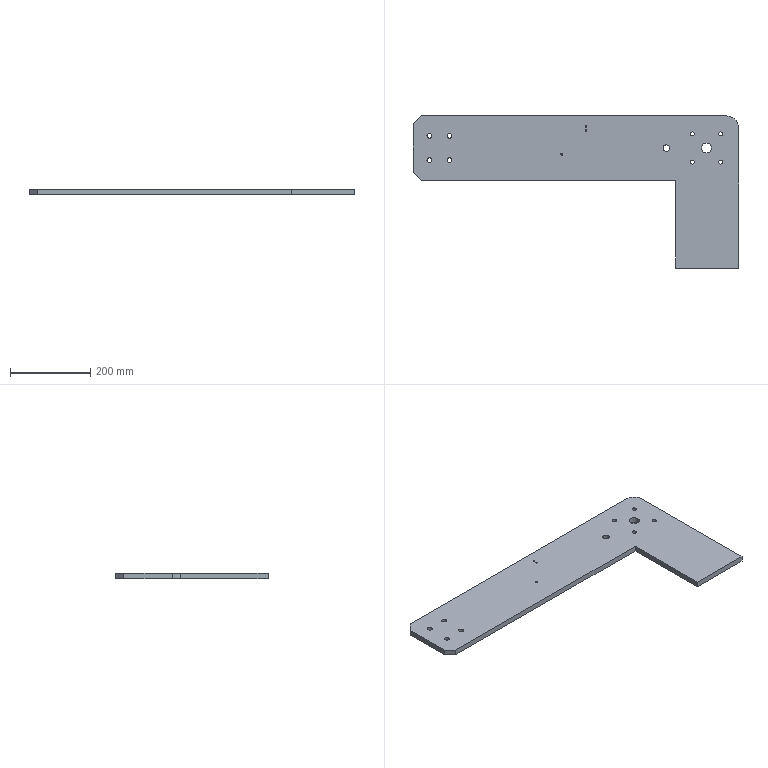Part | STEP file | Head plate 1 | 1 solid | 37 faces | box 810 x 379.049 x 14 mm | volume 2266923 mm3 | cylinder 27 | plane 10 | commonest cylinder face diameters 10 x8 12 x8 4 x4 5 x2 16 x2 25 x2
STEP:
#1=CARTESIAN_POINT('',(312.5,0.,14.));
#2=VERTEX_POINT('',#1);
#3=CARTESIAN_POINT('',(337.5,0.,14.));
#4=VERTEX_POINT('',#3);
#5=CARTESIAN_POINT('',(325.,0.,14.));
#6=DIRECTION('',(0.,0.,1.));
#7=DIRECTION('',(-1.,0.,0.));
#8=AXIS2_PLACEMENT_3D('',#5,#6,#7);
#9=CIRCLE('',#8,12.5);
#10=EDGE_CURVE('',#2,#4,#9,.T.);
#11=ORIENTED_EDGE('',*,*,#10,.T.);
#12=CARTESIAN_POINT('',(337.5,0.,0.));
#13=VERTEX_POINT('',#12);
#14=CARTESIAN_POINT('',(337.5,0.,14.));
#15=DIRECTION('',(0.,0.,-1.));
#16=VECTOR('',#15,1000.);
#17=LINE('',#14,#16);
#18=EDGE_CURVE('',#4,#13,#17,.T.);
#19=ORIENTED_EDGE('',*,*,#18,.T.);
#20=CARTESIAN_POINT('',(312.5,0.,0.));
#21=VERTEX_POINT('',#20);
#22=CARTESIAN_POINT('',(325.,0.,0.));
#23=DIRECTION('',(0.,0.,1.));
#24=DIRECTION('',(-1.,0.,0.));
#25=AXIS2_PLACEMENT_3D('',#22,#23,#24);
#26=CIRCLE('',#25,12.5);
#27=EDGE_CURVE('',#21,#13,#26,.T.);
#28=ORIENTED_EDGE('',*,*,#27,.F.);
#29=CARTESIAN_POINT('',(312.5,0.,14.));
#30=DIRECTION('',(0.,0.,-1.));
#31=VECTOR('',#30,1000.);
#32=LINE('',#29,#31);
#33=EDGE_CURVE('',#2,#21,#32,.T.);
#34=ORIENTED_EDGE('',*,*,#33,.F.);
#35=EDGE_LOOP('',(#11,#19,#28,#34));
#36=FACE_OUTER_BOUND('',#35,.T.);
#37=CARTESIAN_POINT('',(325.,0.,14.));
#38=DIRECTION('',(0.,0.,-1.));
#39=DIRECTION('',(-1.,0.,0.));
#40=AXIS2_PLACEMENT_3D('',#37,#38,#39);
#41=CYLINDRICAL_SURFACE('',#40,12.5);
#42=ADVANCED_FACE('',(#36),#41,.F.);
#43=CARTESIAN_POINT('',(355.,-35.,14.));
#44=VERTEX_POINT('',#43);
#45=CARTESIAN_POINT('',(365.,-35.,14.));
#46=VERTEX_POINT('',#45);
#47=CARTESIAN_POINT('',(360.,-35.,14.));
#48=DIRECTION('',(0.,0.,1.));
#49=DIRECTION('',(-1.,0.,0.));
#50=AXIS2_PLACEMENT_3D('',#47,#48,#49);
#51=CIRCLE('',#50,5.);
#52=EDGE_CURVE('',#44,#46,#51,.T.);
#53=ORIENTED_EDGE('',*,*,#52,.T.);
#54=CARTESIAN_POINT('',(365.,-35.,0.));
#55=VERTEX_POINT('',#54);
#56=CARTESIAN_POINT('',(365.,-35.,14.));
#57=DIRECTION('',(0.,0.,-1.));
#58=VECTOR('',#57,1000.);
#59=LINE('',#56,#58);
#60=EDGE_CURVE('',#46,#55,#59,.T.);
#61=ORIENTED_EDGE('',*,*,#60,.T.);
#62=CARTESIAN_POINT('',(355.,-35.,0.));
#63=VERTEX_POINT('',#62);
#64=CARTESIAN_POINT('',(360.,-35.,0.));
#65=DIRECTION('',(0.,0.,1.));
#66=DIRECTION('',(-1.,0.,0.));
#67=AXIS2_PLACEMENT_3D('',#64,#65,#66);
#68=CIRCLE('',#67,5.);
#69=EDGE_CURVE('',#63,#55,#68,.T.);
#70=ORIENTED_EDGE('',*,*,#69,.F.);
#71=CARTESIAN_POINT('',(355.,-35.,14.));
#72=DIRECTION('',(0.,0.,-1.));
#73=VECTOR('',#72,1000.);
#74=LINE('',#71,#73);
#75=EDGE_CURVE('',#44,#63,#74,.T.);
#76=ORIENTED_EDGE('',*,*,#75,.F.);
#77=EDGE_LOOP('',(#53,#61,#70,#76));
#78=FACE_OUTER_BOUND('',#77,.T.);
#79=CARTESIAN_POINT('',(360.,-35.,14.));
#80=DIRECTION('',(0.,0.,-1.));
#81=DIRECTION('',(-1.,0.,0.));
#82=AXIS2_PLACEMENT_3D('',#79,#80,#81);
#83=CYLINDRICAL_SURFACE('',#82,5.);
#84=ADVANCED_FACE('',(#78),#83,.F.);
#85=CARTESIAN_POINT('',(355.,35.,14.));
#86=VERTEX_POINT('',#85);
#87=CARTESIAN_POINT('',(365.,35.,14.));
#88=VERTEX_POINT('',#87);
#89=CARTESIAN_POINT('',(360.,35.,14.));
#90=DIRECTION('',(0.,0.,1.));
#91=DIRECTION('',(-1.,0.,0.));
#92=AXIS2_PLACEMENT_3D('',#89,#90,#91);
#93=CIRCLE('',#92,5.);
#94=EDGE_CURVE('',#86,#88,#93,.T.);
#95=ORIENTED_EDGE('',*,*,#94,.T.);
#96=CARTESIAN_POINT('',(365.,35.,0.));
#97=VERTEX_POINT('',#96);
#98=CARTESIAN_POINT('',(365.,35.,14.));
#99=DIRECTION('',(0.,0.,-1.));
#100=VECTOR('',#99,1000.);
#101=LINE('',#98,#100);
#102=EDGE_CURVE('',#88,#97,#101,.T.);
#103=ORIENTED_EDGE('',*,*,#102,.T.);
#104=CARTESIAN_POINT('',(355.,35.,0.));
#105=VERTEX_POINT('',#104);
#106=CARTESIAN_POINT('',(360.,35.,0.));
#107=DIRECTION('',(0.,0.,1.));
#108=DIRECTION('',(-1.,0.,0.));
#109=AXIS2_PLACEMENT_3D('',#106,#107,#108);
#110=CIRCLE('',#109,5.);
#111=EDGE_CURVE('',#105,#97,#110,.T.);
#112=ORIENTED_EDGE('',*,*,#111,.F.);
#113=CARTESIAN_POINT('',(355.,35.,14.));
#114=DIRECTION('',(0.,0.,-1.));
#115=VECTOR('',#114,1000.);
#116=LINE('',#113,#115);
#117=EDGE_CURVE('',#86,#105,#116,.T.);
#118=ORIENTED_EDGE('',*,*,#117,.F.);
#119=EDGE_LOOP('',(#95,#103,#112,#118));
#120=FACE_OUTER_BOUND('',#119,.T.);
#121=CARTESIAN_POINT('',(360.,35.,14.));
#122=DIRECTION('',(0.,0.,-1.));
#123=DIRECTION('',(-1.,0.,0.));
#124=AXIS2_PLACEMENT_3D('',#121,#122,#123);
#125=CYLINDRICAL_SURFACE('',#124,5.);
#126=ADVANCED_FACE('',(#120),#125,.F.);
#127=CARTESIAN_POINT('',(285.,35.,14.));
#128=VERTEX_POINT('',#127);
#129=CARTESIAN_POINT('',(295.,35.,14.));
#130=VERTEX_POINT('',#129);
#131=CARTESIAN_POINT('',(290.,35.,14.));
#132=DIRECTION('',(0.,0.,1.));
#133=DIRECTION('',(-1.,0.,0.));
#134=AXIS2_PLACEMENT_3D('',#131,#132,#133);
#135=CIRCLE('',#134,5.);
#136=EDGE_CURVE('',#128,#130,#135,.T.);
#137=ORIENTED_EDGE('',*,*,#136,.T.);
#138=CARTESIAN_POINT('',(295.,35.,0.));
#139=VERTEX_POINT('',#138);
#140=CARTESIAN_POINT('',(295.,35.,14.));
#141=DIRECTION('',(0.,0.,-1.));
#142=VECTOR('',#141,1000.);
#143=LINE('',#140,#142);
#144=EDGE_CURVE('',#130,#139,#143,.T.);
#145=ORIENTED_EDGE('',*,*,#144,.T.);
#146=CARTESIAN_POINT('',(285.,35.,0.));
#147=VERTEX_POINT('',#146);
#148=CARTESIAN_POINT('',(290.,35.,0.));
#149=DIRECTION('',(0.,0.,1.));
#150=DIRECTION('',(-1.,0.,0.));
#151=AXIS2_PLACEMENT_3D('',#148,#149,#150);
#152=CIRCLE('',#151,5.);
#153=EDGE_CURVE('',#147,#139,#152,.T.);
#154=ORIENTED_EDGE('',*,*,#153,.F.);
#155=CARTESIAN_POINT('',(285.,35.,14.));
#156=DIRECTION('',(0.,0.,-1.));
#157=VECTOR('',#156,1000.);
#158=LINE('',#155,#157);
#159=EDGE_CURVE('',#128,#147,#158,.T.);
#160=ORIENTED_EDGE('',*,*,#159,.F.);
#161=EDGE_LOOP('',(#137,#145,#154,#160));
#162=FACE_OUTER_BOUND('',#161,.T.);
#163=CARTESIAN_POINT('',(290.,35.,14.));
#164=DIRECTION('',(0.,0.,-1.));
#165=DIRECTION('',(-1.,0.,0.));
#166=AXIS2_PLACEMENT_3D('',#163,#164,#165);
#167=CYLINDRICAL_SURFACE('',#166,5.);
#168=ADVANCED_FACE('',(#162),#167,.F.);
#169=CARTESIAN_POINT('',(285.,-35.,14.));
#170=VERTEX_POINT('',#169);
#171=CARTESIAN_POINT('',(295.,-35.,14.));
#172=VERTEX_POINT('',#171);
#173=CARTESIAN_POINT('',(290.,-35.,14.));
#174=DIRECTION('',(0.,0.,1.));
#175=DIRECTION('',(-1.,0.,0.));
#176=AXIS2_PLACEMENT_3D('',#173,#174,#175);
#177=CIRCLE('',#176,5.);
#178=EDGE_CURVE('',#170,#172,#177,.T.);
#179=ORIENTED_EDGE('',*,*,#178,.T.);
#180=CARTESIAN_POINT('',(295.,-35.,0.));
#181=VERTEX_POINT('',#180);
#182=CARTESIAN_POINT('',(295.,-35.,14.));
#183=DIRECTION('',(0.,0.,-1.));
#184=VECTOR('',#183,1000.);
#185=LINE('',#182,#184);
#186=EDGE_CURVE('',#172,#181,#185,.T.);
#187=ORIENTED_EDGE('',*,*,#186,.T.);
#188=CARTESIAN_POINT('',(285.,-35.,0.));
#189=VERTEX_POINT('',#188);
#190=CARTESIAN_POINT('',(290.,-35.,0.));
#191=DIRECTION('',(0.,0.,1.));
#192=DIRECTION('',(-1.,0.,0.));
#193=AXIS2_PLACEMENT_3D('',#190,#191,#192);
#194=CIRCLE('',#193,5.);
#195=EDGE_CURVE('',#189,#181,#194,.T.);
#196=ORIENTED_EDGE('',*,*,#195,.F.);
#197=CARTESIAN_POINT('',(285.,-35.,14.));
#198=DIRECTION('',(0.,0.,-1.));
#199=VECTOR('',#198,1000.);
#200=LINE('',#197,#199);
#201=EDGE_CURVE('',#170,#189,#200,.T.);
#202=ORIENTED_EDGE('',*,*,#201,.F.);
#203=EDGE_LOOP('',(#179,#187,#196,#202));
#204=FACE_OUTER_BOUND('',#203,.T.);
#205=CARTESIAN_POINT('',(290.,-35.,14.));
#206=DIRECTION('',(0.,0.,-1.));
#207=DIRECTION('',(-1.,0.,0.));
#208=AXIS2_PLACEMENT_3D('',#205,#206,#207);
#209=CYLINDRICAL_SURFACE('',#208,5.);
#210=ADVANCED_FACE('',(#204),#209,.F.);
#211=CARTESIAN_POINT('',(-37.5,-15.,0.));
#212=VERTEX_POINT('',#211);
#213=CARTESIAN_POINT('',(-32.5,-15.,0.));
#214=VERTEX_POINT('',#213);
#215=CARTESIAN_POINT('',(-35.,-15.,0.));
#216=DIRECTION('',(0.,0.,1.));
#217=DIRECTION('',(1.,0.,0.));
#218=AXIS2_PLACEMENT_3D('',#215,#216,#217);
#219=CIRCLE('',#218,2.5);
#220=EDGE_CURVE('',#212,#214,#219,.T.);
#221=ORIENTED_EDGE('',*,*,#220,.F.);
#222=CARTESIAN_POINT('',(-37.5,-15.,14.));
#223=VERTEX_POINT('',#222);
#224=CARTESIAN_POINT('',(-37.5,-15.,-1.));
#225=DIRECTION('',(0.,0.,1.));
#226=VECTOR('',#225,1000.);
#227=LINE('',#224,#226);
#228=EDGE_CURVE('',#212,#223,#227,.T.);
#229=ORIENTED_EDGE('',*,*,#228,.T.);
#230=CARTESIAN_POINT('',(-32.5,-15.,14.));
#231=VERTEX_POINT('',#230);
#232=CARTESIAN_POINT('',(-35.,-15.,14.));
#233=DIRECTION('',(0.,0.,1.));
#234=DIRECTION('',(1.,0.,0.));
#235=AXIS2_PLACEMENT_3D('',#232,#233,#234);
#236=CIRCLE('',#235,2.5);
#237=EDGE_CURVE('',#223,#231,#236,.T.);
#238=ORIENTED_EDGE('',*,*,#237,.T.);
#239=CARTESIAN_POINT('',(-32.5,-15.,-1.));
#240=DIRECTION('',(0.,0.,1.));
#241=VECTOR('',#240,1000.);
#242=LINE('',#239,#241);
#243=EDGE_CURVE('',#214,#231,#242,.T.);
#244=ORIENTED_EDGE('',*,*,#243,.F.);
#245=EDGE_LOOP('',(#221,#229,#238,#244));
#246=FACE_OUTER_BOUND('',#245,.T.);
#247=CARTESIAN_POINT('',(-35.,-15.,-1.));
#248=DIRECTION('',(0.,0.,1.));
#249=DIRECTION('',(1.,0.,0.));
#250=AXIS2_PLACEMENT_3D('',#247,#248,#249);
#251=CYLINDRICAL_SURFACE('',#250,2.5);
#252=ADVANCED_FACE('',(#246),#251,.F.);
#253=CARTESIAN_POINT('',(-371.,30.,0.));
#254=VERTEX_POINT('',#253);
#255=CARTESIAN_POINT('',(-359.,30.,0.));
#256=VERTEX_POINT('',#255);
#257=CARTESIAN_POINT('',(-365.,30.,0.));
#258=DIRECTION('',(0.,0.,1.));
#259=DIRECTION('',(1.,0.,0.));
#260=AXIS2_PLACEMENT_3D('',#257,#258,#259);
#261=CIRCLE('',#260,6.);
#262=EDGE_CURVE('',#254,#256,#261,.T.);
#263=ORIENTED_EDGE('',*,*,#262,.F.);
#264=CARTESIAN_POINT('',(-371.,30.,14.));
#265=VERTEX_POINT('',#264);
#266=CARTESIAN_POINT('',(-371.,30.,-1.));
#267=DIRECTION('',(0.,0.,1.));
#268=VECTOR('',#267,1000.);
#269=LINE('',#266,#268);
#270=EDGE_CURVE('',#254,#265,#269,.T.);
#271=ORIENTED_EDGE('',*,*,#270,.T.);
#272=CARTESIAN_POINT('',(-359.,30.,14.));
#273=VERTEX_POINT('',#272);
#274=CARTESIAN_POINT('',(-365.,30.,14.));
#275=DIRECTION('',(0.,0.,1.));
#276=DIRECTION('',(1.,0.,0.));
#277=AXIS2_PLACEMENT_3D('',#274,#275,#276);
#278=CIRCLE('',#277,6.);
#279=EDGE_CURVE('',#265,#273,#278,.T.);
#280=ORIENTED_EDGE('',*,*,#279,.T.);
#281=CARTESIAN_POINT('',(-359.,30.,-1.));
#282=DIRECTION('',(0.,0.,1.));
#283=VECTOR('',#282,1000.);
#284=LINE('',#281,#283);
#285=EDGE_CURVE('',#256,#273,#284,.T.);
#286=ORIENTED_EDGE('',*,*,#285,.F.);
#287=EDGE_LOOP('',(#263,#271,#280,#286));
#288=FACE_OUTER_BOUND('',#287,.T.);
#289=CARTESIAN_POINT('',(-365.,30.,-1.));
#290=DIRECTION('',(0.,0.,1.));
#291=DIRECTION('',(1.,0.,0.));
#292=AXIS2_PLACEMENT_3D('',#289,#290,#291);
#293=CYLINDRICAL_SURFACE('',#292,6.);
#294=ADVANCED_FACE('',(#288),#293,.F.);
#295=CARTESIAN_POINT('',(-321.,30.,0.));
#296=VERTEX_POINT('',#295);
#297=CARTESIAN_POINT('',(-309.,30.,0.));
#298=VERTEX_POINT('',#297);
#299=CARTESIAN_POINT('',(-315.,30.,0.));
#300=DIRECTION('',(0.,0.,1.));
#301=DIRECTION('',(1.,0.,0.));
#302=AXIS2_PLACEMENT_3D('',#299,#300,#301);
#303=CIRCLE('',#302,6.);
#304=EDGE_CURVE('',#296,#298,#303,.T.);
#305=ORIENTED_EDGE('',*,*,#304,.F.);
#306=CARTESIAN_POINT('',(-321.,30.,14.));
#307=VERTEX_POINT('',#306);
#308=CARTESIAN_POINT('',(-321.,30.,-1.));
#309=DIRECTION('',(0.,0.,1.));
#310=VECTOR('',#309,1000.);
#311=LINE('',#308,#310);
#312=EDGE_CURVE('',#296,#307,#311,.T.);
#313=ORIENTED_EDGE('',*,*,#312,.T.);
#314=CARTESIAN_POINT('',(-309.,30.,14.));
#315=VERTEX_POINT('',#314);
#316=CARTESIAN_POINT('',(-315.,30.,14.));
#317=DIRECTION('',(0.,0.,1.));
#318=DIRECTION('',(1.,0.,0.));
#319=AXIS2_PLACEMENT_3D('',#316,#317,#318);
#320=CIRCLE('',#319,6.);
#321=EDGE_CURVE('',#307,#315,#320,.T.);
#322=ORIENTED_EDGE('',*,*,#321,.T.);
#323=CARTESIAN_POINT('',(-309.,30.,-1.));
#324=DIRECTION('',(0.,0.,1.));
#325=VECTOR('',#324,1000.);
#326=LINE('',#323,#325);
#327=EDGE_CURVE('',#298,#315,#326,.T.);
#328=ORIENTED_EDGE('',*,*,#327,.F.);
#329=EDGE_LOOP('',(#305,#313,#322,#328));
#330=FACE_OUTER_BOUND('',#329,.T.);
#331=CARTESIAN_POINT('',(-315.,30.,-1.));
#332=DIRECTION('',(0.,0.,1.));
#333=DIRECTION('',(1.,0.,0.));
#334=AXIS2_PLACEMENT_3D('',#331,#332,#333);
#335=CYLINDRICAL_SURFACE('',#334,6.);
#336=ADVANCED_FACE('',(#330),#335,.F.);
#337=CARTESIAN_POINT('',(-371.,-30.,0.));
#338=VERTEX_POINT('',#337);
#339=CARTESIAN_POINT('',(-359.,-30.,0.));
#340=VERTEX_POINT('',#339);
#341=CARTESIAN_POINT('',(-365.,-30.,0.));
#342=DIRECTION('',(0.,0.,1.));
#343=DIRECTION('',(1.,0.,0.));
#344=AXIS2_PLACEMENT_3D('',#341,#342,#343);
#345=CIRCLE('',#344,6.);
#346=EDGE_CURVE('',#338,#340,#345,.T.);
#347=ORIENTED_EDGE('',*,*,#346,.F.);
#348=CARTESIAN_POINT('',(-371.,-30.,14.));
#349=VERTEX_POINT('',#348);
#350=CARTESIAN_POINT('',(-371.,-30.,-1.));
#351=DIRECTION('',(0.,0.,1.));
#352=VECTOR('',#351,1000.);
#353=LINE('',#350,#352);
#354=EDGE_CURVE('',#338,#349,#353,.T.);
#355=ORIENTED_EDGE('',*,*,#354,.T.);
#356=CARTESIAN_POINT('',(-359.,-30.,14.));
#357=VERTEX_POINT('',#356);
#358=CARTESIAN_POINT('',(-365.,-30.,14.));
#359=DIRECTION('',(0.,0.,1.));
#360=DIRECTION('',(1.,0.,0.));
#361=AXIS2_PLACEMENT_3D('',#358,#359,#360);
#362=CIRCLE('',#361,6.);
#363=EDGE_CURVE('',#349,#357,#362,.T.);
#364=ORIENTED_EDGE('',*,*,#363,.T.);
#365=CARTESIAN_POINT('',(-359.,-30.,-1.));
#366=DIRECTION('',(0.,0.,1.));
#367=VECTOR('',#366,1000.);
#368=LINE('',#365,#367);
#369=EDGE_CURVE('',#340,#357,#368,.T.);
#370=ORIENTED_EDGE('',*,*,#369,.F.);
#371=EDGE_LOOP('',(#347,#355,#364,#370));
#372=FACE_OUTER_BOUND('',#371,.T.);
#373=CARTESIAN_POINT('',(-365.,-30.,-1.));
#374=DIRECTION('',(0.,0.,1.));
#375=DIRECTION('',(1.,0.,0.));
#376=AXIS2_PLACEMENT_3D('',#373,#374,#375);
#377=CYLINDRICAL_SURFACE('',#376,6.);
#378=ADVANCED_FACE('',(#372),#377,.F.);
#379=CARTESIAN_POINT('',(-321.,-30.,0.));
#380=VERTEX_POINT('',#379);
#381=CARTESIAN_POINT('',(-309.,-30.,0.));
#382=VERTEX_POINT('',#381);
#383=CARTESIAN_POINT('',(-315.,-30.,0.));
#384=DIRECTION('',(0.,0.,1.));
#385=DIRECTION('',(1.,0.,0.));
#386=AXIS2_PLACEMENT_3D('',#383,#384,#385);
#387=CIRCLE('',#386,6.);
#388=EDGE_CURVE('',#380,#382,#387,.T.);
#389=ORIENTED_EDGE('',*,*,#388,.F.);
#390=CARTESIAN_POINT('',(-321.,-30.,14.));
#391=VERTEX_POINT('',#390);
#392=CARTESIAN_POINT('',(-321.,-30.,-1.));
#393=DIRECTION('',(0.,0.,1.));
#394=VECTOR('',#393,1000.);
#395=LINE('',#392,#394);
#396=EDGE_CURVE('',#380,#391,#395,.T.);
#397=ORIENTED_EDGE('',*,*,#396,.T.);
#398=CARTESIAN_POINT('',(-309.,-30.,14.));
#399=VERTEX_POINT('',#398);
#400=CARTESIAN_POINT('',(-315.,-30.,14.));
#401=DIRECTION('',(0.,0.,1.));
#402=DIRECTION('',(1.,0.,0.));
#403=AXIS2_PLACEMENT_3D('',#400,#401,#402);
#404=CIRCLE('',#403,6.);
#405=EDGE_CURVE('',#391,#399,#404,.T.);
#406=ORIENTED_EDGE('',*,*,#405,.T.);
#407=CARTESIAN_POINT('',(-309.,-30.,-1.));
#408=DIRECTION('',(0.,0.,1.));
#409=VECTOR('',#408,1000.);
#410=LINE('',#407,#409);
#411=EDGE_CURVE('',#382,#399,#410,.T.);
#412=ORIENTED_EDGE('',*,*,#411,.F.);
#413=EDGE_LOOP('',(#389,#397,#406,#412));
#414=FACE_OUTER_BOUND('',#413,.T.);
#415=CARTESIAN_POINT('',(-315.,-30.,-1.));
#416=DIRECTION('',(0.,0.,1.));
#417=DIRECTION('',(1.,0.,0.));
#418=AXIS2_PLACEMENT_3D('',#415,#416,#417);
#419=CYLINDRICAL_SURFACE('',#418,6.);
#420=ADVANCED_FACE('',(#414),#419,.F.);
#421=CARTESIAN_POINT('',(23.,54.,14.));
#422=VERTEX_POINT('',#421);
#423=CARTESIAN_POINT('',(27.,54.,14.));
#424=VERTEX_POINT('',#423);
#425=CARTESIAN_POINT('',(25.,54.,14.));
#426=DIRECTION('',(0.,0.,1.));
#427=DIRECTION('',(-1.,0.,0.));
#428=AXIS2_PLACEMENT_3D('',#425,#426,#427);
#429=CIRCLE('',#428,2.);
#430=EDGE_CURVE('',#422,#424,#429,.T.);
#431=ORIENTED_EDGE('',*,*,#430,.T.);
#432=CARTESIAN_POINT('',(27.,54.,0.));
#433=VERTEX_POINT('',#432);
#434=CARTESIAN_POINT('',(27.,54.,20.));
#435=DIRECTION('',(0.,0.,-1.));
#436=VECTOR('',#435,1000.);
#437=LINE('',#434,#436);
#438=EDGE_CURVE('',#424,#433,#437,.T.);
#439=ORIENTED_EDGE('',*,*,#438,.T.);
#440=CARTESIAN_POINT('',(23.,54.,0.));
#441=VERTEX_POINT('',#440);
#442=CARTESIAN_POINT('',(25.,54.,0.));
#443=DIRECTION('',(0.,0.,1.));
#444=DIRECTION('',(-1.,0.,0.));
#445=AXIS2_PLACEMENT_3D('',#442,#443,#444);
#446=CIRCLE('',#445,2.);
#447=EDGE_CURVE('',#441,#433,#446,.T.);
#448=ORIENTED_EDGE('',*,*,#447,.F.);
#449=CARTESIAN_POINT('',(23.,54.,20.));
#450=DIRECTION('',(0.,0.,-1.));
#451=VECTOR('',#450,1000.);
#452=LINE('',#449,#451);
#453=EDGE_CURVE('',#422,#441,#452,.T.);
#454=ORIENTED_EDGE('',*,*,#453,.F.);
#455=EDGE_LOOP('',(#431,#439,#448,#454));
#456=FACE_OUTER_BOUND('',#455,.T.);
#457=CARTESIAN_POINT('',(25.,54.,20.));
#458=DIRECTION('',(0.,0.,-1.));
#459=DIRECTION('',(-1.,0.,0.));
#460=AXIS2_PLACEMENT_3D('',#457,#458,#459);
#461=CYLINDRICAL_SURFACE('',#460,2.);
#462=ADVANCED_FACE('',(#456),#461,.F.);
#463=CARTESIAN_POINT('',(23.,44.,14.));
#464=VERTEX_POINT('',#463);
#465=CARTESIAN_POINT('',(27.,44.,14.));
#466=VERTEX_POINT('',#465);
#467=CARTESIAN_POINT('',(25.,44.,14.));
#468=DIRECTION('',(0.,0.,1.));
#469=DIRECTION('',(-1.,0.,0.));
#470=AXIS2_PLACEMENT_3D('',#467,#468,#469);
#471=CIRCLE('',#470,2.);
#472=EDGE_CURVE('',#464,#466,#471,.T.);
#473=ORIENTED_EDGE('',*,*,#472,.T.);
#474=CARTESIAN_POINT('',(27.,44.,0.));
#475=VERTEX_POINT('',#474);
#476=CARTESIAN_POINT('',(27.,44.,20.));
#477=DIRECTION('',(0.,0.,-1.));
#478=VECTOR('',#477,1000.);
#479=LINE('',#476,#478);
#480=EDGE_CURVE('',#466,#475,#479,.T.);
#481=ORIENTED_EDGE('',*,*,#480,.T.);
#482=CARTESIAN_POINT('',(23.,44.,0.));
#483=VERTEX_POINT('',#482);
#484=CARTESIAN_POINT('',(25.,44.,0.));
#485=DIRECTION('',(0.,0.,1.));
#486=DIRECTION('',(-1.,0.,0.));
#487=AXIS2_PLACEMENT_3D('',#484,#485,#486);
#488=CIRCLE('',#487,2.);
#489=EDGE_CURVE('',#483,#475,#488,.T.);
#490=ORIENTED_EDGE('',*,*,#489,.F.);
#491=CARTESIAN_POINT('',(23.,44.,20.));
#492=DIRECTION('',(0.,0.,-1.));
#493=VECTOR('',#492,1000.);
#494=LINE('',#491,#493);
#495=EDGE_CURVE('',#464,#483,#494,.T.);
#496=ORIENTED_EDGE('',*,*,#495,.F.);
#497=EDGE_LOOP('',(#473,#481,#490,#496));
#498=FACE_OUTER_BOUND('',#497,.T.);
#499=CARTESIAN_POINT('',(25.,44.,20.));
#500=DIRECTION('',(0.,0.,-1.));
#501=DIRECTION('',(-1.,0.,0.));
#502=AXIS2_PLACEMENT_3D('',#499,#500,#501);
#503=CYLINDRICAL_SURFACE('',#502,2.);
#504=ADVANCED_FACE('',(#498),#503,.F.);
#505=CARTESIAN_POINT('',(217.,0.,14.));
#506=VERTEX_POINT('',#505);
#507=CARTESIAN_POINT('',(233.,0.,14.));
#508=VERTEX_POINT('',#507);
#509=CARTESIAN_POINT('',(225.,0.,14.));
#510=DIRECTION('',(0.,0.,1.));
#511=DIRECTION('',(-1.,0.,0.));
#512=AXIS2_PLACEMENT_3D('',#509,#510,#511);
#513=CIRCLE('',#512,8.);
#514=EDGE_CURVE('',#506,#508,#513,.T.);
#515=ORIENTED_EDGE('',*,*,#514,.T.);
#516=CARTESIAN_POINT('',(233.,0.,0.));
#517=VERTEX_POINT('',#516);
#518=CARTESIAN_POINT('',(233.,0.,15.));
#519=DIRECTION('',(0.,0.,-1.));
#520=VECTOR('',#519,1000.);
#521=LINE('',#518,#520);
#522=EDGE_CURVE('',#508,#517,#521,.T.);
#523=ORIENTED_EDGE('',*,*,#522,.T.);
#524=CARTESIAN_POINT('',(217.,0.,0.));
#525=VERTEX_POINT('',#524);
#526=CARTESIAN_POINT('',(225.,0.,0.));
#527=DIRECTION('',(0.,0.,1.));
#528=DIRECTION('',(-1.,0.,0.));
#529=AXIS2_PLACEMENT_3D('',#526,#527,#528);
#530=CIRCLE('',#529,8.);
#531=EDGE_CURVE('',#525,#517,#530,.T.);
#532=ORIENTED_EDGE('',*,*,#531,.F.);
#533=CARTESIAN_POINT('',(217.,0.,15.));
#534=DIRECTION('',(0.,0.,-1.));
#535=VECTOR('',#534,1000.);
#536=LINE('',#533,#535);
#537=EDGE_CURVE('',#506,#525,#536,.T.);
#538=ORIENTED_EDGE('',*,*,#537,.F.);
#539=EDGE_LOOP('',(#515,#523,#532,#538));
#540=FACE_OUTER_BOUND('',#539,.T.);
#541=CARTESIAN_POINT('',(225.,0.,15.));
#542=DIRECTION('',(0.,0.,-1.));
#543=DIRECTION('',(-1.,0.,0.));
#544=AXIS2_PLACEMENT_3D('',#541,#542,#543);
#545=CYLINDRICAL_SURFACE('',#544,8.);
#546=ADVANCED_FACE('',(#540),#545,.F.);
#547=CARTESIAN_POINT('',(-385.,-80.,14.));
#548=VERTEX_POINT('',#547);
#549=CARTESIAN_POINT('',(-405.,-60.,14.));
#550=VERTEX_POINT('',#549);
#551=CARTESIAN_POINT('',(-385.,-80.,14.));
#552=DIRECTION('',(-0.7071,0.7071,0.));
#553=VECTOR('',#552,1000.);
#554=LINE('',#551,#553);
#555=EDGE_CURVE('',#548,#550,#554,.T.);
#556=ORIENTED_EDGE('',*,*,#555,.F.);
#557=CARTESIAN_POINT('',(247.869,-80.,14.));
#558=VERTEX_POINT('',#557);
#559=CARTESIAN_POINT('',(405.,-80.,14.));
#560=DIRECTION('',(-1.,0.,0.));
#561=VECTOR('',#560,1000.);
#562=LINE('',#559,#561);
#563=EDGE_CURVE('',#558,#548,#562,.T.);
#564=ORIENTED_EDGE('',*,*,#563,.F.);
#565=CARTESIAN_POINT('',(247.869,-299.049,14.));
#566=VERTEX_POINT('',#565);
#567=CARTESIAN_POINT('',(247.869,-80.,14.));
#568=DIRECTION('',(0.,-1.,0.));
#569=VECTOR('',#568,1000.);
#570=LINE('',#567,#569);
#571=EDGE_CURVE('',#558,#566,#570,.T.);
#572=ORIENTED_EDGE('',*,*,#571,.T.);
#573=CARTESIAN_POINT('',(405.,-299.049,14.));
#574=VERTEX_POINT('',#573);
#575=CARTESIAN_POINT('',(247.869,-299.049,14.));
#576=DIRECTION('',(1.,0.,0.));
#577=VECTOR('',#576,1000.);
#578=LINE('',#575,#577);
#579=EDGE_CURVE('',#566,#574,#578,.T.);
#580=ORIENTED_EDGE('',*,*,#579,.T.);
#581=CARTESIAN_POINT('',(405.,50.,14.));
#582=VERTEX_POINT('',#581);
#583=CARTESIAN_POINT('',(405.,-80.,14.));
#584=DIRECTION('',(0.,-1.,0.));
#585=VECTOR('',#584,1000.);
#586=LINE('',#583,#585);
#587=EDGE_CURVE('',#582,#574,#586,.T.);
#588=ORIENTED_EDGE('',*,*,#587,.F.);
#589=CARTESIAN_POINT('',(375.,80.,14.));
#590=VERTEX_POINT('',#589);
#591=CARTESIAN_POINT('',(375.,50.,14.));
#592=DIRECTION('',(0.,0.,-1.));
#593=DIRECTION('',(-1.,0.,0.));
#594=AXIS2_PLACEMENT_3D('',#591,#592,#593);
#595=CIRCLE('',#594,30.);
#596=EDGE_CURVE('',#590,#582,#595,.T.);
#597=ORIENTED_EDGE('',*,*,#596,.F.);
#598=CARTESIAN_POINT('',(-385.,80.,14.));
#599=VERTEX_POINT('',#598);
#600=CARTESIAN_POINT('',(405.,80.,14.));
#601=DIRECTION('',(1.,0.,0.));
#602=VECTOR('',#601,1000.);
#603=LINE('',#600,#602);
#604=EDGE_CURVE('',#599,#590,#603,.T.);
#605=ORIENTED_EDGE('',*,*,#604,.F.);
#606=CARTESIAN_POINT('',(-405.,60.,14.));
#607=VERTEX_POINT('',#606);
#608=CARTESIAN_POINT('',(-405.,60.,14.));
#609=DIRECTION('',(0.7071,0.7071,0.));
#610=VECTOR('',#609,1000.);
#611=LINE('',#608,#610);
#612=EDGE_CURVE('',#607,#599,#611,.T.);
#613=ORIENTED_EDGE('',*,*,#612,.F.);
#614=CARTESIAN_POINT('',(-405.,-80.,14.));
#615=DIRECTION('',(0.,1.,0.));
#616=VECTOR('',#615,1000.);
#617=LINE('',#614,#616);
#618=EDGE_CURVE('',#550,#607,#617,.T.);
#619=ORIENTED_EDGE('',*,*,#618,.F.);
#620=EDGE_LOOP('',(#556,#564,#572,#580,#588,#597,#605,#613,#619));
#621=FACE_OUTER_BOUND('',#620,.T.);
#622=ORIENTED_EDGE('',*,*,#10,.F.);
#623=CARTESIAN_POINT('',(325.,0.,14.));
#624=DIRECTION('',(0.,0.,1.));
#625=DIRECTION('',(-1.,0.,0.));
#626=AXIS2_PLACEMENT_3D('',#623,#624,#625);
#627=CIRCLE('',#626,12.5);
#628=EDGE_CURVE('',#4,#2,#627,.T.);
#629=ORIENTED_EDGE('',*,*,#628,.F.);
#630=EDGE_LOOP('',(#622,#629));
#631=FACE_BOUND('',#630,.T.);
#632=ORIENTED_EDGE('',*,*,#52,.F.);
#633=CARTESIAN_POINT('',(360.,-35.,14.));
#634=DIRECTION('',(0.,0.,1.));
#635=DIRECTION('',(-1.,0.,0.));
#636=AXIS2_PLACEMENT_3D('',#633,#634,#635);
#637=CIRCLE('',#636,5.);
#638=EDGE_CURVE('',#46,#44,#637,.T.);
#639=ORIENTED_EDGE('',*,*,#638,.F.);
#640=EDGE_LOOP('',(#632,#639));
#641=FACE_BOUND('',#640,.T.);
#642=ORIENTED_EDGE('',*,*,#94,.F.);
#643=CARTESIAN_POINT('',(360.,35.,14.));
#644=DIRECTION('',(0.,0.,1.));
#645=DIRECTION('',(-1.,0.,0.));
#646=AXIS2_PLACEMENT_3D('',#643,#644,#645);
#647=CIRCLE('',#646,5.);
#648=EDGE_CURVE('',#88,#86,#647,.T.);
#649=ORIENTED_EDGE('',*,*,#648,.F.);
#650=EDGE_LOOP('',(#642,#649));
#651=FACE_BOUND('',#650,.T.);
#652=ORIENTED_EDGE('',*,*,#136,.F.);
#653=CARTESIAN_POINT('',(290.,35.,14.));
#654=DIRECTION('',(0.,0.,1.));
#655=DIRECTION('',(-1.,0.,0.));
#656=AXIS2_PLACEMENT_3D('',#653,#654,#655);
#657=CIRCLE('',#656,5.);
#658=EDGE_CURVE('',#130,#128,#657,.T.);
#659=ORIENTED_EDGE('',*,*,#658,.F.);
#660=EDGE_LOOP('',(#652,#659));
#661=FACE_BOUND('',#660,.T.);
#662=ORIENTED_EDGE('',*,*,#178,.F.);
#663=CARTESIAN_POINT('',(290.,-35.,14.));
#664=DIRECTION('',(0.,0.,1.));
#665=DIRECTION('',(-1.,0.,0.));
#666=AXIS2_PLACEMENT_3D('',#663,#664,#665);
#667=CIRCLE('',#666,5.);
#668=EDGE_CURVE('',#172,#170,#667,.T.);
#669=ORIENTED_EDGE('',*,*,#668,.F.);
#670=EDGE_LOOP('',(#662,#669));
#671=FACE_BOUND('',#670,.T.);
#672=CARTESIAN_POINT('',(-35.,-15.,14.));
#673=DIRECTION('',(0.,0.,1.));
#674=DIRECTION('',(1.,0.,0.));
#675=AXIS2_PLACEMENT_3D('',#672,#673,#674);
#676=CIRCLE('',#675,2.5);
#677=EDGE_CURVE('',#231,#223,#676,.T.);
#678=ORIENTED_EDGE('',*,*,#677,.F.);
#679=ORIENTED_EDGE('',*,*,#237,.F.);
#680=EDGE_LOOP('',(#678,#679));
#681=FACE_BOUND('',#680,.T.);
#682=CARTESIAN_POINT('',(-365.,30.,14.));
#683=DIRECTION('',(0.,0.,1.));
#684=DIRECTION('',(1.,0.,0.));
#685=AXIS2_PLACEMENT_3D('',#682,#683,#684);
#686=CIRCLE('',#685,6.);
#687=EDGE_CURVE('',#273,#265,#686,.T.);
#688=ORIENTED_EDGE('',*,*,#687,.F.);
#689=ORIENTED_EDGE('',*,*,#279,.F.);
#690=EDGE_LOOP('',(#688,#689));
#691=FACE_BOUND('',#690,.T.);
#692=CARTESIAN_POINT('',(-315.,30.,14.));
#693=DIRECTION('',(0.,0.,1.));
#694=DIRECTION('',(1.,0.,0.));
#695=AXIS2_PLACEMENT_3D('',#692,#693,#694);
#696=CIRCLE('',#695,6.);
#697=EDGE_CURVE('',#315,#307,#696,.T.);
#698=ORIENTED_EDGE('',*,*,#697,.F.);
#699=ORIENTED_EDGE('',*,*,#321,.F.);
#700=EDGE_LOOP('',(#698,#699));
#701=FACE_BOUND('',#700,.T.);
#702=CARTESIAN_POINT('',(-365.,-30.,14.));
#703=DIRECTION('',(0.,0.,1.));
#704=DIRECTION('',(1.,0.,0.));
#705=AXIS2_PLACEMENT_3D('',#702,#703,#704);
#706=CIRCLE('',#705,6.);
#707=EDGE_CURVE('',#357,#349,#706,.T.);
#708=ORIENTED_EDGE('',*,*,#707,.F.);
#709=ORIENTED_EDGE('',*,*,#363,.F.);
#710=EDGE_LOOP('',(#708,#709));
#711=FACE_BOUND('',#710,.T.);
#712=CARTESIAN_POINT('',(-315.,-30.,14.));
#713=DIRECTION('',(0.,0.,1.));
#714=DIRECTION('',(1.,0.,0.));
#715=AXIS2_PLACEMENT_3D('',#712,#713,#714);
#716=CIRCLE('',#715,6.);
#717=EDGE_CURVE('',#399,#391,#716,.T.);
#718=ORIENTED_EDGE('',*,*,#717,.F.);
#719=ORIENTED_EDGE('',*,*,#405,.F.);
#720=EDGE_LOOP('',(#718,#719));
#721=FACE_BOUND('',#720,.T.);
#722=ORIENTED_EDGE('',*,*,#430,.F.);
#723=CARTESIAN_POINT('',(25.,54.,14.));
#724=DIRECTION('',(0.,0.,1.));
#725=DIRECTION('',(-1.,0.,0.));
#726=AXIS2_PLACEMENT_3D('',#723,#724,#725);
#727=CIRCLE('',#726,2.);
#728=EDGE_CURVE('',#424,#422,#727,.T.);
#729=ORIENTED_EDGE('',*,*,#728,.F.);
#730=EDGE_LOOP('',(#722,#729));
#731=FACE_BOUND('',#730,.T.);
#732=ORIENTED_EDGE('',*,*,#472,.F.);
#733=CARTESIAN_POINT('',(25.,44.,14.));
#734=DIRECTION('',(0.,0.,1.));
#735=DIRECTION('',(-1.,0.,0.));
#736=AXIS2_PLACEMENT_3D('',#733,#734,#735);
#737=CIRCLE('',#736,2.);
#738=EDGE_CURVE('',#466,#464,#737,.T.);
#739=ORIENTED_EDGE('',*,*,#738,.F.);
#740=EDGE_LOOP('',(#732,#739));
#741=FACE_BOUND('',#740,.T.);
#742=ORIENTED_EDGE('',*,*,#514,.F.);
#743=CARTESIAN_POINT('',(225.,0.,14.));
#744=DIRECTION('',(0.,0.,1.));
#745=DIRECTION('',(-1.,0.,0.));
#746=AXIS2_PLACEMENT_3D('',#743,#744,#745);
#747=CIRCLE('',#746,8.);
#748=EDGE_CURVE('',#508,#506,#747,.T.);
#749=ORIENTED_EDGE('',*,*,#748,.F.);
#750=EDGE_LOOP('',(#742,#749));
#751=FACE_BOUND('',#750,.T.);
#752=CARTESIAN_POINT('',(405.,-80.,14.));
#753=DIRECTION('',(0.,0.,-1.));
#754=DIRECTION('',(-1.,0.,0.));
#755=AXIS2_PLACEMENT_3D('',#752,#753,#754);
#756=PLANE('',#755);
#757=ADVANCED_FACE('',(#621,#631,#641,#651,#661,#671,#681,#691,#701,#711,#721,#731,#741,#751),#756,.F.);
#758=CARTESIAN_POINT('',(-405.,-60.,0.));
#759=VERTEX_POINT('',#758);
#760=CARTESIAN_POINT('',(-405.,-60.,14.));
#761=DIRECTION('',(0.,0.,-1.));
#762=VECTOR('',#761,1000.);
#763=LINE('',#760,#762);
#764=EDGE_CURVE('',#550,#759,#763,.T.);
#765=ORIENTED_EDGE('',*,*,#764,.F.);
#766=ORIENTED_EDGE('',*,*,#618,.T.);
#767=CARTESIAN_POINT('',(-405.,60.,0.));
#768=VERTEX_POINT('',#767);
#769=CARTESIAN_POINT('',(-405.,60.,14.));
#770=DIRECTION('',(0.,0.,1.));
#771=VECTOR('',#770,1000.);
#772=LINE('',#769,#771);
#773=EDGE_CURVE('',#768,#607,#772,.T.);
#774=ORIENTED_EDGE('',*,*,#773,.F.);
#775=CARTESIAN_POINT('',(-405.,80.,0.));
#776=DIRECTION('',(0.,1.,0.));
#777=VECTOR('',#776,1000.);
#778=LINE('',#775,#777);
#779=EDGE_CURVE('',#759,#768,#778,.T.);
#780=ORIENTED_EDGE('',*,*,#779,.F.);
#781=EDGE_LOOP('',(#765,#766,#774,#780));
#782=FACE_OUTER_BOUND('',#781,.T.);
#783=CARTESIAN_POINT('',(-405.,80.,14.));
#784=DIRECTION('',(1.,0.,0.));
#785=DIRECTION('',(0.,0.,-1.));
#786=AXIS2_PLACEMENT_3D('',#783,#784,#785);
#787=PLANE('',#786);
#788=ADVANCED_FACE('',(#782),#787,.F.);
#789=ORIENTED_EDGE('',*,*,#764,.T.);
#790=CARTESIAN_POINT('',(-385.,-80.,0.));
#791=VERTEX_POINT('',#790);
#792=CARTESIAN_POINT('',(-385.,-80.,0.));
#793=DIRECTION('',(-0.7071,0.7071,0.));
#794=VECTOR('',#793,1000.);
#795=LINE('',#792,#794);
#796=EDGE_CURVE('',#791,#759,#795,.T.);
#797=ORIENTED_EDGE('',*,*,#796,.F.);
#798=CARTESIAN_POINT('',(-385.,-80.,14.));
#799=DIRECTION('',(0.,0.,-1.));
#800=VECTOR('',#799,1000.);
#801=LINE('',#798,#800);
#802=EDGE_CURVE('',#548,#791,#801,.T.);
#803=ORIENTED_EDGE('',*,*,#802,.F.);
#804=ORIENTED_EDGE('',*,*,#555,.T.);
#805=EDGE_LOOP('',(#789,#797,#803,#804));
#806=FACE_OUTER_BOUND('',#805,.T.);
#807=CARTESIAN_POINT('',(-385.,-80.,14.));
#808=DIRECTION('',(0.7071,0.7071,0.));
#809=DIRECTION('',(-0.7071,0.7071,0.));
#810=AXIS2_PLACEMENT_3D('',#807,#808,#809);
#811=PLANE('',#810);
#812=ADVANCED_FACE('',(#806),#811,.F.);
#813=CARTESIAN_POINT('',(247.869,-80.,0.));
#814=VERTEX_POINT('',#813);
#815=CARTESIAN_POINT('',(405.,-80.,0.));
#816=DIRECTION('',(-1.,0.,0.));
#817=VECTOR('',#816,1000.);
#818=LINE('',#815,#817);
#819=EDGE_CURVE('',#814,#791,#818,.T.);
#820=ORIENTED_EDGE('',*,*,#819,.F.);
#821=CARTESIAN_POINT('',(247.869,-80.,-294.475));
#822=DIRECTION('',(0.,0.,1.));
#823=VECTOR('',#822,1000.);
#824=LINE('',#821,#823);
#825=EDGE_CURVE('',#814,#558,#824,.T.);
#826=ORIENTED_EDGE('',*,*,#825,.T.);
#827=ORIENTED_EDGE('',*,*,#563,.T.);
#828=ORIENTED_EDGE('',*,*,#802,.T.);
#829=EDGE_LOOP('',(#820,#826,#827,#828));
#830=FACE_OUTER_BOUND('',#829,.T.);
#831=CARTESIAN_POINT('',(405.,-80.,14.));
#832=DIRECTION('',(0.,1.,0.));
#833=DIRECTION('',(-1.,0.,0.));
#834=AXIS2_PLACEMENT_3D('',#831,#832,#833);
#835=PLANE('',#834);
#836=ADVANCED_FACE('',(#830),#835,.F.);
#837=ORIENTED_EDGE('',*,*,#587,.T.);
#838=CARTESIAN_POINT('',(405.,-299.049,0.));
#839=VERTEX_POINT('',#838);
#840=CARTESIAN_POINT('',(405.,-299.049,-294.475));
#841=DIRECTION('',(0.,0.,1.));
#842=VECTOR('',#841,1000.);
#843=LINE('',#840,#842);
#844=EDGE_CURVE('',#839,#574,#843,.T.);
#845=ORIENTED_EDGE('',*,*,#844,.F.);
#846=CARTESIAN_POINT('',(405.,50.,0.));
#847=VERTEX_POINT('',#846);
#848=CARTESIAN_POINT('',(405.,80.,0.));
#849=DIRECTION('',(0.,-1.,0.));
#850=VECTOR('',#849,1000.);
#851=LINE('',#848,#850);
#852=EDGE_CURVE('',#847,#839,#851,.T.);
#853=ORIENTED_EDGE('',*,*,#852,.F.);
#854=CARTESIAN_POINT('',(405.,50.,14.));
#855=DIRECTION('',(0.,0.,-1.));
#856=VECTOR('',#855,1000.);
#857=LINE('',#854,#856);
#858=EDGE_CURVE('',#582,#847,#857,.T.);
#859=ORIENTED_EDGE('',*,*,#858,.F.);
#860=EDGE_LOOP('',(#837,#845,#853,#859));
#861=FACE_OUTER_BOUND('',#860,.T.);
#862=CARTESIAN_POINT('',(405.,80.,14.));
#863=DIRECTION('',(-1.,0.,0.));
#864=DIRECTION('',(0.,0.,1.));
#865=AXIS2_PLACEMENT_3D('',#862,#863,#864);
#866=PLANE('',#865);
#867=ADVANCED_FACE('',(#861),#866,.F.);
#868=CARTESIAN_POINT('',(375.,80.,0.));
#869=VERTEX_POINT('',#868);
#870=CARTESIAN_POINT('',(375.,50.,0.));
#871=DIRECTION('',(0.,0.,1.));
#872=DIRECTION('',(-1.,0.,0.));
#873=AXIS2_PLACEMENT_3D('',#870,#871,#872);
#874=CIRCLE('',#873,30.);
#875=EDGE_CURVE('',#847,#869,#874,.T.);
#876=ORIENTED_EDGE('',*,*,#875,.T.);
#877=CARTESIAN_POINT('',(375.,80.,14.));
#878=DIRECTION('',(0.,0.,1.));
#879=VECTOR('',#878,1000.);
#880=LINE('',#877,#879);
#881=EDGE_CURVE('',#869,#590,#880,.T.);
#882=ORIENTED_EDGE('',*,*,#881,.T.);
#883=ORIENTED_EDGE('',*,*,#596,.T.);
#884=ORIENTED_EDGE('',*,*,#858,.T.);
#885=EDGE_LOOP('',(#876,#882,#883,#884));
#886=FACE_OUTER_BOUND('',#885,.T.);
#887=CARTESIAN_POINT('',(375.,50.,14.));
#888=DIRECTION('',(0.,0.,-1.));
#889=DIRECTION('',(-1.,0.,0.));
#890=AXIS2_PLACEMENT_3D('',#887,#888,#889);
#891=CYLINDRICAL_SURFACE('',#890,30.);
#892=ADVANCED_FACE('',(#886),#891,.T.);
#893=CARTESIAN_POINT('',(-385.,80.,0.));
#894=VERTEX_POINT('',#893);
#895=CARTESIAN_POINT('',(-385.,80.,14.));
#896=DIRECTION('',(0.,0.,-1.));
#897=VECTOR('',#896,1000.);
#898=LINE('',#895,#897);
#899=EDGE_CURVE('',#599,#894,#898,.T.);
#900=ORIENTED_EDGE('',*,*,#899,.F.);
#901=ORIENTED_EDGE('',*,*,#604,.T.);
#902=ORIENTED_EDGE('',*,*,#881,.F.);
#903=CARTESIAN_POINT('',(405.,80.,0.));
#904=DIRECTION('',(1.,0.,0.));
#905=VECTOR('',#904,1000.);
#906=LINE('',#903,#905);
#907=EDGE_CURVE('',#894,#869,#906,.T.);
#908=ORIENTED_EDGE('',*,*,#907,.F.);
#909=EDGE_LOOP('',(#900,#901,#902,#908));
#910=FACE_OUTER_BOUND('',#909,.T.);
#911=CARTESIAN_POINT('',(405.,80.,14.));
#912=DIRECTION('',(0.,-1.,0.));
#913=DIRECTION('',(1.,0.,0.));
#914=AXIS2_PLACEMENT_3D('',#911,#912,#913);
#915=PLANE('',#914);
#916=ADVANCED_FACE('',(#910),#915,.F.);
#917=ORIENTED_EDGE('',*,*,#899,.T.);
#918=CARTESIAN_POINT('',(-405.,60.,0.));
#919=DIRECTION('',(0.7071,0.7071,0.));
#920=VECTOR('',#919,1000.);
#921=LINE('',#918,#920);
#922=EDGE_CURVE('',#768,#894,#921,.T.);
#923=ORIENTED_EDGE('',*,*,#922,.F.);
#924=ORIENTED_EDGE('',*,*,#773,.T.);
#925=ORIENTED_EDGE('',*,*,#612,.T.);
#926=EDGE_LOOP('',(#917,#923,#924,#925));
#927=FACE_OUTER_BOUND('',#926,.T.);
#928=CARTESIAN_POINT('',(-405.,60.,14.));
#929=DIRECTION('',(0.7071,-0.7071,0.));
#930=DIRECTION('',(0.7071,0.7071,0.));
#931=AXIS2_PLACEMENT_3D('',#928,#929,#930);
#932=PLANE('',#931);
#933=ADVANCED_FACE('',(#927),#932,.F.);
#934=ORIENTED_EDGE('',*,*,#18,.F.);
#935=ORIENTED_EDGE('',*,*,#628,.T.);
#936=ORIENTED_EDGE('',*,*,#33,.T.);
#937=CARTESIAN_POINT('',(325.,0.,0.));
#938=DIRECTION('',(0.,0.,1.));
#939=DIRECTION('',(-1.,0.,0.));
#940=AXIS2_PLACEMENT_3D('',#937,#938,#939);
#941=CIRCLE('',#940,12.5);
#942=EDGE_CURVE('',#13,#21,#941,.T.);
#943=ORIENTED_EDGE('',*,*,#942,.F.);
#944=EDGE_LOOP('',(#934,#935,#936,#943));
#945=FACE_OUTER_BOUND('',#944,.T.);
#946=CARTESIAN_POINT('',(325.,0.,14.));
#947=DIRECTION('',(0.,0.,-1.));
#948=DIRECTION('',(-1.,0.,0.));
#949=AXIS2_PLACEMENT_3D('',#946,#947,#948);
#950=CYLINDRICAL_SURFACE('',#949,12.5);
#951=ADVANCED_FACE('',(#945),#950,.F.);
#952=ORIENTED_EDGE('',*,*,#60,.F.);
#953=ORIENTED_EDGE('',*,*,#638,.T.);
#954=ORIENTED_EDGE('',*,*,#75,.T.);
#955=CARTESIAN_POINT('',(360.,-35.,0.));
#956=DIRECTION('',(0.,0.,1.));
#957=DIRECTION('',(-1.,0.,0.));
#958=AXIS2_PLACEMENT_3D('',#955,#956,#957);
#959=CIRCLE('',#958,5.);
#960=EDGE_CURVE('',#55,#63,#959,.T.);
#961=ORIENTED_EDGE('',*,*,#960,.F.);
#962=EDGE_LOOP('',(#952,#953,#954,#961));
#963=FACE_OUTER_BOUND('',#962,.T.);
#964=CARTESIAN_POINT('',(360.,-35.,14.));
#965=DIRECTION('',(0.,0.,-1.));
#966=DIRECTION('',(-1.,0.,0.));
#967=AXIS2_PLACEMENT_3D('',#964,#965,#966);
#968=CYLINDRICAL_SURFACE('',#967,5.);
#969=ADVANCED_FACE('',(#963),#968,.F.);
#970=ORIENTED_EDGE('',*,*,#102,.F.);
#971=ORIENTED_EDGE('',*,*,#648,.T.);
#972=ORIENTED_EDGE('',*,*,#117,.T.);
#973=CARTESIAN_POINT('',(360.,35.,0.));
#974=DIRECTION('',(0.,0.,1.));
#975=DIRECTION('',(-1.,0.,0.));
#976=AXIS2_PLACEMENT_3D('',#973,#974,#975);
#977=CIRCLE('',#976,5.);
#978=EDGE_CURVE('',#97,#105,#977,.T.);
#979=ORIENTED_EDGE('',*,*,#978,.F.);
#980=EDGE_LOOP('',(#970,#971,#972,#979));
#981=FACE_OUTER_BOUND('',#980,.T.);
#982=CARTESIAN_POINT('',(360.,35.,14.));
#983=DIRECTION('',(0.,0.,-1.));
#984=DIRECTION('',(-1.,0.,0.));
#985=AXIS2_PLACEMENT_3D('',#982,#983,#984);
#986=CYLINDRICAL_SURFACE('',#985,5.);
#987=ADVANCED_FACE('',(#981),#986,.F.);
#988=ORIENTED_EDGE('',*,*,#144,.F.);
#989=ORIENTED_EDGE('',*,*,#658,.T.);
#990=ORIENTED_EDGE('',*,*,#159,.T.);
#991=CARTESIAN_POINT('',(290.,35.,0.));
#992=DIRECTION('',(0.,0.,1.));
#993=DIRECTION('',(-1.,0.,0.));
#994=AXIS2_PLACEMENT_3D('',#991,#992,#993);
#995=CIRCLE('',#994,5.);
#996=EDGE_CURVE('',#139,#147,#995,.T.);
#997=ORIENTED_EDGE('',*,*,#996,.F.);
#998=EDGE_LOOP('',(#988,#989,#990,#997));
#999=FACE_OUTER_BOUND('',#998,.T.);
#1000=CARTESIAN_POINT('',(290.,35.,14.));
#1001=DIRECTION('',(0.,0.,-1.));
#1002=DIRECTION('',(-1.,0.,0.));
#1003=AXIS2_PLACEMENT_3D('',#1000,#1001,#1002);
#1004=CYLINDRICAL_SURFACE('',#1003,5.);
#1005=ADVANCED_FACE('',(#999),#1004,.F.);
#1006=ORIENTED_EDGE('',*,*,#186,.F.);
#1007=ORIENTED_EDGE('',*,*,#668,.T.);
#1008=ORIENTED_EDGE('',*,*,#201,.T.);
#1009=CARTESIAN_POINT('',(290.,-35.,0.));
#1010=DIRECTION('',(0.,0.,1.));
#1011=DIRECTION('',(-1.,0.,0.));
#1012=AXIS2_PLACEMENT_3D('',#1009,#1010,#1011);
#1013=CIRCLE('',#1012,5.);
#1014=EDGE_CURVE('',#181,#189,#1013,.T.);
#1015=ORIENTED_EDGE('',*,*,#1014,.F.);
#1016=EDGE_LOOP('',(#1006,#1007,#1008,#1015));
#1017=FACE_OUTER_BOUND('',#1016,.T.);
#1018=CARTESIAN_POINT('',(290.,-35.,14.));
#1019=DIRECTION('',(0.,0.,-1.));
#1020=DIRECTION('',(-1.,0.,0.));
#1021=AXIS2_PLACEMENT_3D('',#1018,#1019,#1020);
#1022=CYLINDRICAL_SURFACE('',#1021,5.);
#1023=ADVANCED_FACE('',(#1017),#1022,.F.);
#1024=ORIENTED_EDGE('',*,*,#228,.F.);
#1025=CARTESIAN_POINT('',(-35.,-15.,0.));
#1026=DIRECTION('',(0.,0.,1.));
#1027=DIRECTION('',(1.,0.,0.));
#1028=AXIS2_PLACEMENT_3D('',#1025,#1026,#1027);
#1029=CIRCLE('',#1028,2.5);
#1030=EDGE_CURVE('',#214,#212,#1029,.T.);
#1031=ORIENTED_EDGE('',*,*,#1030,.F.);
#1032=ORIENTED_EDGE('',*,*,#243,.T.);
#1033=ORIENTED_EDGE('',*,*,#677,.T.);
#1034=EDGE_LOOP('',(#1024,#1031,#1032,#1033));
#1035=FACE_OUTER_BOUND('',#1034,.T.);
#1036=CARTESIAN_POINT('',(-35.,-15.,-1.));
#1037=DIRECTION('',(0.,0.,1.));
#1038=DIRECTION('',(1.,0.,0.));
#1039=AXIS2_PLACEMENT_3D('',#1036,#1037,#1038);
#1040=CYLINDRICAL_SURFACE('',#1039,2.5);
#1041=ADVANCED_FACE('',(#1035),#1040,.F.);
#1042=ORIENTED_EDGE('',*,*,#270,.F.);
#1043=CARTESIAN_POINT('',(-365.,30.,0.));
#1044=DIRECTION('',(0.,0.,1.));
#1045=DIRECTION('',(1.,0.,0.));
#1046=AXIS2_PLACEMENT_3D('',#1043,#1044,#1045);
#1047=CIRCLE('',#1046,6.);
#1048=EDGE_CURVE('',#256,#254,#1047,.T.);
#1049=ORIENTED_EDGE('',*,*,#1048,.F.);
#1050=ORIENTED_EDGE('',*,*,#285,.T.);
#1051=ORIENTED_EDGE('',*,*,#687,.T.);
#1052=EDGE_LOOP('',(#1042,#1049,#1050,#1051));
#1053=FACE_OUTER_BOUND('',#1052,.T.);
#1054=CARTESIAN_POINT('',(-365.,30.,-1.));
#1055=DIRECTION('',(0.,0.,1.));
#1056=DIRECTION('',(1.,0.,0.));
#1057=AXIS2_PLACEMENT_3D('',#1054,#1055,#1056);
#1058=CYLINDRICAL_SURFACE('',#1057,6.);
#1059=ADVANCED_FACE('',(#1053),#1058,.F.);
#1060=ORIENTED_EDGE('',*,*,#312,.F.);
#1061=CARTESIAN_POINT('',(-315.,30.,0.));
#1062=DIRECTION('',(0.,0.,1.));
#1063=DIRECTION('',(1.,0.,0.));
#1064=AXIS2_PLACEMENT_3D('',#1061,#1062,#1063);
#1065=CIRCLE('',#1064,6.);
#1066=EDGE_CURVE('',#298,#296,#1065,.T.);
#1067=ORIENTED_EDGE('',*,*,#1066,.F.);
#1068=ORIENTED_EDGE('',*,*,#327,.T.);
#1069=ORIENTED_EDGE('',*,*,#697,.T.);
#1070=EDGE_LOOP('',(#1060,#1067,#1068,#1069));
#1071=FACE_OUTER_BOUND('',#1070,.T.);
#1072=CARTESIAN_POINT('',(-315.,30.,-1.));
#1073=DIRECTION('',(0.,0.,1.));
#1074=DIRECTION('',(1.,0.,0.));
#1075=AXIS2_PLACEMENT_3D('',#1072,#1073,#1074);
#1076=CYLINDRICAL_SURFACE('',#1075,6.);
#1077=ADVANCED_FACE('',(#1071),#1076,.F.);
#1078=ORIENTED_EDGE('',*,*,#354,.F.);
#1079=CARTESIAN_POINT('',(-365.,-30.,0.));
#1080=DIRECTION('',(0.,0.,1.));
#1081=DIRECTION('',(1.,0.,0.));
#1082=AXIS2_PLACEMENT_3D('',#1079,#1080,#1081);
#1083=CIRCLE('',#1082,6.);
#1084=EDGE_CURVE('',#340,#338,#1083,.T.);
#1085=ORIENTED_EDGE('',*,*,#1084,.F.);
#1086=ORIENTED_EDGE('',*,*,#369,.T.);
#1087=ORIENTED_EDGE('',*,*,#707,.T.);
#1088=EDGE_LOOP('',(#1078,#1085,#1086,#1087));
#1089=FACE_OUTER_BOUND('',#1088,.T.);
#1090=CARTESIAN_POINT('',(-365.,-30.,-1.));
#1091=DIRECTION('',(0.,0.,1.));
#1092=DIRECTION('',(1.,0.,0.));
#1093=AXIS2_PLACEMENT_3D('',#1090,#1091,#1092);
#1094=CYLINDRICAL_SURFACE('',#1093,6.);
#1095=ADVANCED_FACE('',(#1089),#1094,.F.);
#1096=ORIENTED_EDGE('',*,*,#396,.F.);
#1097=CARTESIAN_POINT('',(-315.,-30.,0.));
#1098=DIRECTION('',(0.,0.,1.));
#1099=DIRECTION('',(1.,0.,0.));
#1100=AXIS2_PLACEMENT_3D('',#1097,#1098,#1099);
#1101=CIRCLE('',#1100,6.);
#1102=EDGE_CURVE('',#382,#380,#1101,.T.);
#1103=ORIENTED_EDGE('',*,*,#1102,.F.);
#1104=ORIENTED_EDGE('',*,*,#411,.T.);
#1105=ORIENTED_EDGE('',*,*,#717,.T.);
#1106=EDGE_LOOP('',(#1096,#1103,#1104,#1105));
#1107=FACE_OUTER_BOUND('',#1106,.T.);
#1108=CARTESIAN_POINT('',(-315.,-30.,-1.));
#1109=DIRECTION('',(0.,0.,1.));
#1110=DIRECTION('',(1.,0.,0.));
#1111=AXIS2_PLACEMENT_3D('',#1108,#1109,#1110);
#1112=CYLINDRICAL_SURFACE('',#1111,6.);
#1113=ADVANCED_FACE('',(#1107),#1112,.F.);
#1114=ORIENTED_EDGE('',*,*,#438,.F.);
#1115=ORIENTED_EDGE('',*,*,#728,.T.);
#1116=ORIENTED_EDGE('',*,*,#453,.T.);
#1117=CARTESIAN_POINT('',(25.,54.,0.));
#1118=DIRECTION('',(0.,0.,1.));
#1119=DIRECTION('',(-1.,0.,0.));
#1120=AXIS2_PLACEMENT_3D('',#1117,#1118,#1119);
#1121=CIRCLE('',#1120,2.);
#1122=EDGE_CURVE('',#433,#441,#1121,.T.);
#1123=ORIENTED_EDGE('',*,*,#1122,.F.);
#1124=EDGE_LOOP('',(#1114,#1115,#1116,#1123));
#1125=FACE_OUTER_BOUND('',#1124,.T.);
#1126=CARTESIAN_POINT('',(25.,54.,20.));
#1127=DIRECTION('',(0.,0.,-1.));
#1128=DIRECTION('',(-1.,0.,0.));
#1129=AXIS2_PLACEMENT_3D('',#1126,#1127,#1128);
#1130=CYLINDRICAL_SURFACE('',#1129,2.);
#1131=ADVANCED_FACE('',(#1125),#1130,.F.);
#1132=ORIENTED_EDGE('',*,*,#480,.F.);
#1133=ORIENTED_EDGE('',*,*,#738,.T.);
#1134=ORIENTED_EDGE('',*,*,#495,.T.);
#1135=CARTESIAN_POINT('',(25.,44.,0.));
#1136=DIRECTION('',(0.,0.,1.));
#1137=DIRECTION('',(-1.,0.,0.));
#1138=AXIS2_PLACEMENT_3D('',#1135,#1136,#1137);
#1139=CIRCLE('',#1138,2.);
#1140=EDGE_CURVE('',#475,#483,#1139,.T.);
#1141=ORIENTED_EDGE('',*,*,#1140,.F.);
#1142=EDGE_LOOP('',(#1132,#1133,#1134,#1141));
#1143=FACE_OUTER_BOUND('',#1142,.T.);
#1144=CARTESIAN_POINT('',(25.,44.,20.));
#1145=DIRECTION('',(0.,0.,-1.));
#1146=DIRECTION('',(-1.,0.,0.));
#1147=AXIS2_PLACEMENT_3D('',#1144,#1145,#1146);
#1148=CYLINDRICAL_SURFACE('',#1147,2.);
#1149=ADVANCED_FACE('',(#1143),#1148,.F.);
#1150=ORIENTED_EDGE('',*,*,#522,.F.);
#1151=ORIENTED_EDGE('',*,*,#748,.T.);
#1152=ORIENTED_EDGE('',*,*,#537,.T.);
#1153=CARTESIAN_POINT('',(225.,0.,0.));
#1154=DIRECTION('',(0.,0.,1.));
#1155=DIRECTION('',(-1.,0.,0.));
#1156=AXIS2_PLACEMENT_3D('',#1153,#1154,#1155);
#1157=CIRCLE('',#1156,8.);
#1158=EDGE_CURVE('',#517,#525,#1157,.T.);
#1159=ORIENTED_EDGE('',*,*,#1158,.F.);
#1160=EDGE_LOOP('',(#1150,#1151,#1152,#1159));
#1161=FACE_OUTER_BOUND('',#1160,.T.);
#1162=CARTESIAN_POINT('',(225.,0.,15.));
#1163=DIRECTION('',(0.,0.,-1.));
#1164=DIRECTION('',(-1.,0.,0.));
#1165=AXIS2_PLACEMENT_3D('',#1162,#1163,#1164);
#1166=CYLINDRICAL_SURFACE('',#1165,8.);
#1167=ADVANCED_FACE('',(#1161),#1166,.F.);
#1168=ORIENTED_EDGE('',*,*,#852,.T.);
#1169=CARTESIAN_POINT('',(247.869,-299.049,0.));
#1170=VERTEX_POINT('',#1169);
#1171=CARTESIAN_POINT('',(247.869,-299.049,0.));
#1172=DIRECTION('',(1.,0.,0.));
#1173=VECTOR('',#1172,1000.);
#1174=LINE('',#1171,#1173);
#1175=EDGE_CURVE('',#1170,#839,#1174,.T.);
#1176=ORIENTED_EDGE('',*,*,#1175,.F.);
#1177=CARTESIAN_POINT('',(247.869,-80.,0.));
#1178=DIRECTION('',(0.,-1.,0.));
#1179=VECTOR('',#1178,1000.);
#1180=LINE('',#1177,#1179);
#1181=EDGE_CURVE('',#814,#1170,#1180,.T.);
#1182=ORIENTED_EDGE('',*,*,#1181,.F.);
#1183=ORIENTED_EDGE('',*,*,#819,.T.);
#1184=ORIENTED_EDGE('',*,*,#796,.T.);
#1185=ORIENTED_EDGE('',*,*,#779,.T.);
#1186=ORIENTED_EDGE('',*,*,#922,.T.);
#1187=ORIENTED_EDGE('',*,*,#907,.T.);
#1188=ORIENTED_EDGE('',*,*,#875,.F.);
#1189=EDGE_LOOP('',(#1168,#1176,#1182,#1183,#1184,#1185,#1186,#1187,#1188));
#1190=FACE_OUTER_BOUND('',#1189,.T.);
#1191=ORIENTED_EDGE('',*,*,#27,.T.);
#1192=ORIENTED_EDGE('',*,*,#942,.T.);
#1193=EDGE_LOOP('',(#1191,#1192));
#1194=FACE_BOUND('',#1193,.T.);
#1195=ORIENTED_EDGE('',*,*,#69,.T.);
#1196=ORIENTED_EDGE('',*,*,#960,.T.);
#1197=EDGE_LOOP('',(#1195,#1196));
#1198=FACE_BOUND('',#1197,.T.);
#1199=ORIENTED_EDGE('',*,*,#111,.T.);
#1200=ORIENTED_EDGE('',*,*,#978,.T.);
#1201=EDGE_LOOP('',(#1199,#1200));
#1202=FACE_BOUND('',#1201,.T.);
#1203=ORIENTED_EDGE('',*,*,#153,.T.);
#1204=ORIENTED_EDGE('',*,*,#996,.T.);
#1205=EDGE_LOOP('',(#1203,#1204));
#1206=FACE_BOUND('',#1205,.T.);
#1207=ORIENTED_EDGE('',*,*,#195,.T.);
#1208=ORIENTED_EDGE('',*,*,#1014,.T.);
#1209=EDGE_LOOP('',(#1207,#1208));
#1210=FACE_BOUND('',#1209,.T.);
#1211=ORIENTED_EDGE('',*,*,#1030,.T.);
#1212=ORIENTED_EDGE('',*,*,#220,.T.);
#1213=EDGE_LOOP('',(#1211,#1212));
#1214=FACE_BOUND('',#1213,.T.);
#1215=ORIENTED_EDGE('',*,*,#1048,.T.);
#1216=ORIENTED_EDGE('',*,*,#262,.T.);
#1217=EDGE_LOOP('',(#1215,#1216));
#1218=FACE_BOUND('',#1217,.T.);
#1219=ORIENTED_EDGE('',*,*,#1066,.T.);
#1220=ORIENTED_EDGE('',*,*,#304,.T.);
#1221=EDGE_LOOP('',(#1219,#1220));
#1222=FACE_BOUND('',#1221,.T.);
#1223=ORIENTED_EDGE('',*,*,#1084,.T.);
#1224=ORIENTED_EDGE('',*,*,#346,.T.);
#1225=EDGE_LOOP('',(#1223,#1224));
#1226=FACE_BOUND('',#1225,.T.);
#1227=ORIENTED_EDGE('',*,*,#1102,.T.);
#1228=ORIENTED_EDGE('',*,*,#388,.T.);
#1229=EDGE_LOOP('',(#1227,#1228));
#1230=FACE_BOUND('',#1229,.T.);
#1231=ORIENTED_EDGE('',*,*,#447,.T.);
#1232=ORIENTED_EDGE('',*,*,#1122,.T.);
#1233=EDGE_LOOP('',(#1231,#1232));
#1234=FACE_BOUND('',#1233,.T.);
#1235=ORIENTED_EDGE('',*,*,#489,.T.);
#1236=ORIENTED_EDGE('',*,*,#1140,.T.);
#1237=EDGE_LOOP('',(#1235,#1236));
#1238=FACE_BOUND('',#1237,.T.);
#1239=ORIENTED_EDGE('',*,*,#531,.T.);
#1240=ORIENTED_EDGE('',*,*,#1158,.T.);
#1241=EDGE_LOOP('',(#1239,#1240));
#1242=FACE_BOUND('',#1241,.T.);
#1243=CARTESIAN_POINT('',(405.,-80.,0.));
#1244=DIRECTION('',(0.,0.,-1.));
#1245=DIRECTION('',(-1.,0.,0.));
#1246=AXIS2_PLACEMENT_3D('',#1243,#1244,#1245);
#1247=PLANE('',#1246);
#1248=ADVANCED_FACE('',(#1190,#1194,#1198,#1202,#1206,#1210,#1214,#1218,#1222,#1226,#1230,#1234,#1238,#1242),#1247,.T.);
#1249=ORIENTED_EDGE('',*,*,#825,.F.);
#1250=ORIENTED_EDGE('',*,*,#1181,.T.);
#1251=CARTESIAN_POINT('',(247.869,-299.049,-294.475));
#1252=DIRECTION('',(0.,0.,1.));
#1253=VECTOR('',#1252,1000.);
#1254=LINE('',#1251,#1253);
#1255=EDGE_CURVE('',#1170,#566,#1254,.T.);
#1256=ORIENTED_EDGE('',*,*,#1255,.T.);
#1257=ORIENTED_EDGE('',*,*,#571,.F.);
#1258=EDGE_LOOP('',(#1249,#1250,#1256,#1257));
#1259=FACE_OUTER_BOUND('',#1258,.T.);
#1260=CARTESIAN_POINT('',(247.869,-80.,-294.475));
#1261=DIRECTION('',(-1.,0.,0.));
#1262=DIRECTION('',(0.,0.,1.));
#1263=AXIS2_PLACEMENT_3D('',#1260,#1261,#1262);
#1264=PLANE('',#1263);
#1265=ADVANCED_FACE('',(#1259),#1264,.T.);
#1266=ORIENTED_EDGE('',*,*,#1255,.F.);
#1267=ORIENTED_EDGE('',*,*,#1175,.T.);
#1268=ORIENTED_EDGE('',*,*,#844,.T.);
#1269=ORIENTED_EDGE('',*,*,#579,.F.);
#1270=EDGE_LOOP('',(#1266,#1267,#1268,#1269));
#1271=FACE_OUTER_BOUND('',#1270,.T.);
#1272=CARTESIAN_POINT('',(247.869,-299.049,-294.475));
#1273=DIRECTION('',(0.,-1.,0.));
#1274=DIRECTION('',(0.,0.,-1.));
#1275=AXIS2_PLACEMENT_3D('',#1272,#1273,#1274);
#1276=PLANE('',#1275);
#1277=ADVANCED_FACE('',(#1271),#1276,.T.);
#1278=CLOSED_SHELL('',(#42,#84,#126,#168,#210,#252,#294,#336,#378,#420,#462,#504,#546,#757,#788,#812,#836,#867,#892,#916,#933,#951,#969,#987,#1005,#1023,#1041,#1059,#1077,#1095,#1113,#1131,#1149,#1167,#1248,#1265,#1277));
#1279=MANIFOLD_SOLID_BREP('',#1278);
#1280=CARTESIAN_POINT('',(0.,0.,0.));
#1281=DIRECTION('',(0.,0.,1.));
#1282=DIRECTION('',(1.,0.,0.));
#1283=AXIS2_PLACEMENT_3D('',#1280,#1281,#1282);
#1284=(LENGTH_UNIT()NAMED_UNIT(*)SI_UNIT(.MILLI.,.METRE.));
#1285=UNCERTAINTY_MEASURE_WITH_UNIT(LENGTH_MEASURE(0.00001),#1284,'','');
#1286=(NAMED_UNIT(*)PLANE_ANGLE_UNIT()SI_UNIT($,.RADIAN.));
#1287=(NAMED_UNIT(*)SI_UNIT($,.STERADIAN.)SOLID_ANGLE_UNIT());
#1288=(GEOMETRIC_REPRESENTATION_CONTEXT(3)GLOBAL_UNCERTAINTY_ASSIGNED_CONTEXT((#1285))GLOBAL_UNIT_ASSIGNED_CONTEXT((#1284,#1286,#1287))REPRESENTATION_CONTEXT('',''));
#1289=ADVANCED_BREP_SHAPE_REPRESENTATION('',(#1279,#1283),#1288);